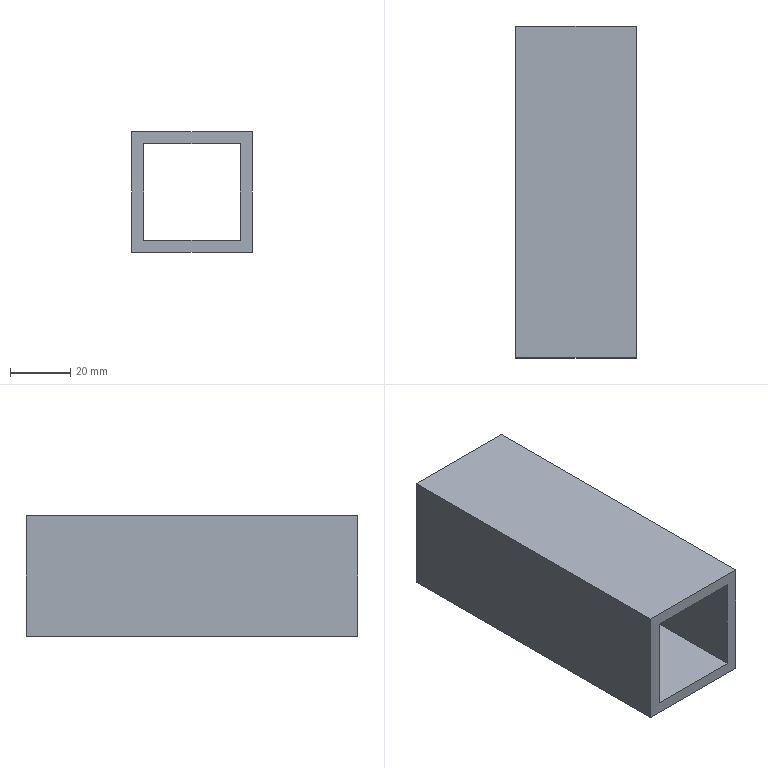Part | NX | features solid 2 | 1 solid | 10 faces | box 40 x 110 x 40 mm | volume 63360 mm3 | plane 10
STEP:
#1=CARTESIAN_POINT('',(1100.,-330.,-85.));
#2=VERTEX_POINT('',#1);
#3=CARTESIAN_POINT('',(1100.,-220.,-85.));
#4=VERTEX_POINT('',#3);
#5=CARTESIAN_POINT('',(1100.,1629.393,-85.));
#6=DIRECTION('',(0.,1.,0.));
#7=VECTOR('',#6,1000.);
#8=LINE('',#5,#7);
#9=EDGE_CURVE('',#2,#4,#8,.T.);
#10=ORIENTED_EDGE('',*,*,#9,.F.);
#11=CARTESIAN_POINT('',(1100.,-330.,-45.));
#12=VERTEX_POINT('',#11);
#13=CARTESIAN_POINT('',(1100.,-330.,-70.));
#14=DIRECTION('',(0.,0.,1.));
#15=VECTOR('',#14,1000.);
#16=LINE('',#13,#15);
#17=EDGE_CURVE('',#2,#12,#16,.T.);
#18=ORIENTED_EDGE('',*,*,#17,.T.);
#19=CARTESIAN_POINT('',(1100.,-220.,-45.));
#20=VERTEX_POINT('',#19);
#21=CARTESIAN_POINT('',(1100.,1714.393,-45.));
#22=DIRECTION('',(0.,1.,0.));
#23=VECTOR('',#22,1000.);
#24=LINE('',#21,#23);
#25=EDGE_CURVE('',#12,#20,#24,.T.);
#26=ORIENTED_EDGE('',*,*,#25,.T.);
#27=CARTESIAN_POINT('',(1100.,-220.,-70.));
#28=DIRECTION('',(0.,0.,1.));
#29=VECTOR('',#28,1000.);
#30=LINE('',#27,#29);
#31=EDGE_CURVE('',#4,#20,#30,.T.);
#32=ORIENTED_EDGE('',*,*,#31,.F.);
#33=EDGE_LOOP('',(#10,#18,#26,#32));
#34=FACE_BOUND('',#33,.T.);
#35=CARTESIAN_POINT('',(1100.,1629.393,-70.));
#36=DIRECTION('',(1.,0.,0.));
#37=DIRECTION('',(0.,0.,1.));
#38=AXIS2_PLACEMENT_3D('',#35,#36,#37);
#39=PLANE('',#38);
#40=ADVANCED_FACE('',(#34),#39,.F.);
#41=CARTESIAN_POINT('',(1140.,-330.,-85.));
#42=VERTEX_POINT('',#41);
#43=CARTESIAN_POINT('',(1140.,-220.,-85.));
#44=VERTEX_POINT('',#43);
#45=CARTESIAN_POINT('',(1140.,1714.393,-85.));
#46=DIRECTION('',(0.,1.,0.));
#47=VECTOR('',#46,1000.);
#48=LINE('',#45,#47);
#49=EDGE_CURVE('',#42,#44,#48,.T.);
#50=ORIENTED_EDGE('',*,*,#49,.F.);
#51=CARTESIAN_POINT('',(520.,-330.,-85.));
#52=DIRECTION('',(-1.,0.,0.));
#53=VECTOR('',#52,1000.);
#54=LINE('',#51,#53);
#55=EDGE_CURVE('',#42,#2,#54,.T.);
#56=ORIENTED_EDGE('',*,*,#55,.T.);
#57=ORIENTED_EDGE('',*,*,#9,.T.);
#58=CARTESIAN_POINT('',(520.,-220.,-85.));
#59=DIRECTION('',(-1.,0.,0.));
#60=VECTOR('',#59,1000.);
#61=LINE('',#58,#60);
#62=EDGE_CURVE('',#44,#4,#61,.T.);
#63=ORIENTED_EDGE('',*,*,#62,.F.);
#64=EDGE_LOOP('',(#50,#56,#57,#63));
#65=FACE_BOUND('',#64,.T.);
#66=CARTESIAN_POINT('',(520.,1714.393,-85.));
#67=DIRECTION('',(0.,0.,1.));
#68=DIRECTION('',(-1.,0.,0.));
#69=AXIS2_PLACEMENT_3D('',#66,#67,#68);
#70=PLANE('',#69);
#71=ADVANCED_FACE('',(#65),#70,.F.);
#72=ORIENTED_EDGE('',*,*,#25,.F.);
#73=CARTESIAN_POINT('',(1140.,-330.,-45.));
#74=VERTEX_POINT('',#73);
#75=CARTESIAN_POINT('',(480.,-330.,-45.));
#76=DIRECTION('',(1.,0.,0.));
#77=VECTOR('',#76,1000.);
#78=LINE('',#75,#77);
#79=EDGE_CURVE('',#12,#74,#78,.T.);
#80=ORIENTED_EDGE('',*,*,#79,.T.);
#81=CARTESIAN_POINT('',(1140.,-220.,-45.));
#82=VERTEX_POINT('',#81);
#83=CARTESIAN_POINT('',(1140.,1714.393,-45.));
#84=DIRECTION('',(0.,-1.,0.));
#85=VECTOR('',#84,1000.);
#86=LINE('',#83,#85);
#87=EDGE_CURVE('',#82,#74,#86,.T.);
#88=ORIENTED_EDGE('',*,*,#87,.F.);
#89=CARTESIAN_POINT('',(480.,-220.,-45.));
#90=DIRECTION('',(1.,0.,0.));
#91=VECTOR('',#90,1000.);
#92=LINE('',#89,#91);
#93=EDGE_CURVE('',#20,#82,#92,.T.);
#94=ORIENTED_EDGE('',*,*,#93,.F.);
#95=EDGE_LOOP('',(#72,#80,#88,#94));
#96=FACE_BOUND('',#95,.T.);
#97=CARTESIAN_POINT('',(480.,1714.393,-45.));
#98=DIRECTION('',(0.,0.,-1.));
#99=DIRECTION('',(1.,0.,0.));
#100=AXIS2_PLACEMENT_3D('',#97,#98,#99);
#101=PLANE('',#100);
#102=ADVANCED_FACE('',(#96),#101,.F.);
#103=ORIENTED_EDGE('',*,*,#87,.T.);
#104=CARTESIAN_POINT('',(1140.,-330.,-40.));
#105=DIRECTION('',(0.,0.,-1.));
#106=VECTOR('',#105,1000.);
#107=LINE('',#104,#106);
#108=EDGE_CURVE('',#74,#42,#107,.T.);
#109=ORIENTED_EDGE('',*,*,#108,.T.);
#110=ORIENTED_EDGE('',*,*,#49,.T.);
#111=CARTESIAN_POINT('',(1140.,-220.,-40.));
#112=DIRECTION('',(0.,0.,-1.));
#113=VECTOR('',#112,1000.);
#114=LINE('',#111,#113);
#115=EDGE_CURVE('',#82,#44,#114,.T.);
#116=ORIENTED_EDGE('',*,*,#115,.F.);
#117=EDGE_LOOP('',(#103,#109,#110,#116));
#118=FACE_BOUND('',#117,.T.);
#119=CARTESIAN_POINT('',(1140.,1629.393,-40.));
#120=DIRECTION('',(-1.,0.,0.));
#121=DIRECTION('',(0.,0.,-1.));
#122=AXIS2_PLACEMENT_3D('',#119,#120,#121);
#123=PLANE('',#122);
#124=ADVANCED_FACE('',(#118),#123,.F.);
#125=CARTESIAN_POINT('',(1104.,-330.,-81.));
#126=VERTEX_POINT('',#125);
#127=CARTESIAN_POINT('',(1104.,-330.,-49.));
#128=VERTEX_POINT('',#127);
#129=CARTESIAN_POINT('',(1104.,-330.,-70.));
#130=DIRECTION('',(0.,0.,1.));
#131=VECTOR('',#130,1000.);
#132=LINE('',#129,#131);
#133=EDGE_CURVE('',#126,#128,#132,.T.);
#134=ORIENTED_EDGE('',*,*,#133,.T.);
#135=CARTESIAN_POINT('',(1136.,-330.,-49.));
#136=VERTEX_POINT('',#135);
#137=CARTESIAN_POINT('',(480.,-330.,-49.));
#138=DIRECTION('',(1.,0.,0.));
#139=VECTOR('',#138,1000.);
#140=LINE('',#137,#139);
#141=EDGE_CURVE('',#128,#136,#140,.T.);
#142=ORIENTED_EDGE('',*,*,#141,.T.);
#143=CARTESIAN_POINT('',(1136.,-330.,-81.));
#144=VERTEX_POINT('',#143);
#145=CARTESIAN_POINT('',(1136.,-330.,-40.));
#146=DIRECTION('',(0.,0.,-1.));
#147=VECTOR('',#146,1000.);
#148=LINE('',#145,#147);
#149=EDGE_CURVE('',#136,#144,#148,.T.);
#150=ORIENTED_EDGE('',*,*,#149,.T.);
#151=CARTESIAN_POINT('',(520.,-330.,-81.));
#152=DIRECTION('',(-1.,0.,0.));
#153=VECTOR('',#152,1000.);
#154=LINE('',#151,#153);
#155=EDGE_CURVE('',#144,#126,#154,.T.);
#156=ORIENTED_EDGE('',*,*,#155,.T.);
#157=EDGE_LOOP('',(#134,#142,#150,#156));
#158=FACE_BOUND('',#157,.T.);
#159=ORIENTED_EDGE('',*,*,#55,.F.);
#160=ORIENTED_EDGE('',*,*,#108,.F.);
#161=ORIENTED_EDGE('',*,*,#79,.F.);
#162=ORIENTED_EDGE('',*,*,#17,.F.);
#163=EDGE_LOOP('',(#159,#160,#161,#162));
#164=FACE_BOUND('',#163,.T.);
#165=CARTESIAN_POINT('',(1250.,-330.,-45.));
#166=DIRECTION('',(0.,-1.,0.));
#167=DIRECTION('',(0.,0.,-1.));
#168=AXIS2_PLACEMENT_3D('',#165,#166,#167);
#169=PLANE('',#168);
#170=ADVANCED_FACE('',(#158,#164),#169,.T.);
#171=CARTESIAN_POINT('',(1104.,-220.,-81.));
#172=VERTEX_POINT('',#171);
#173=CARTESIAN_POINT('',(1104.,-220.,-49.));
#174=VERTEX_POINT('',#173);
#175=CARTESIAN_POINT('',(1104.,-220.,-70.));
#176=DIRECTION('',(0.,0.,1.));
#177=VECTOR('',#176,1000.);
#178=LINE('',#175,#177);
#179=EDGE_CURVE('',#172,#174,#178,.T.);
#180=ORIENTED_EDGE('',*,*,#179,.T.);
#181=CARTESIAN_POINT('',(1104.,1714.393,-49.));
#182=DIRECTION('',(0.,1.,0.));
#183=VECTOR('',#182,1000.);
#184=LINE('',#181,#183);
#185=EDGE_CURVE('',#128,#174,#184,.T.);
#186=ORIENTED_EDGE('',*,*,#185,.F.);
#187=ORIENTED_EDGE('',*,*,#133,.F.);
#188=CARTESIAN_POINT('',(1104.,1629.393,-81.));
#189=DIRECTION('',(0.,1.,0.));
#190=VECTOR('',#189,1000.);
#191=LINE('',#188,#190);
#192=EDGE_CURVE('',#126,#172,#191,.T.);
#193=ORIENTED_EDGE('',*,*,#192,.T.);
#194=EDGE_LOOP('',(#180,#186,#187,#193));
#195=FACE_BOUND('',#194,.T.);
#196=CARTESIAN_POINT('',(1104.,1629.393,-70.));
#197=DIRECTION('',(1.,0.,0.));
#198=DIRECTION('',(0.,0.,1.));
#199=AXIS2_PLACEMENT_3D('',#196,#197,#198);
#200=PLANE('',#199);
#201=ADVANCED_FACE('',(#195),#200,.T.);
#202=CARTESIAN_POINT('',(1136.,-220.,-81.));
#203=VERTEX_POINT('',#202);
#204=CARTESIAN_POINT('',(520.,-220.,-81.));
#205=DIRECTION('',(-1.,0.,0.));
#206=VECTOR('',#205,1000.);
#207=LINE('',#204,#206);
#208=EDGE_CURVE('',#203,#172,#207,.T.);
#209=ORIENTED_EDGE('',*,*,#208,.T.);
#210=ORIENTED_EDGE('',*,*,#192,.F.);
#211=ORIENTED_EDGE('',*,*,#155,.F.);
#212=CARTESIAN_POINT('',(1136.,1714.393,-81.));
#213=DIRECTION('',(0.,1.,0.));
#214=VECTOR('',#213,1000.);
#215=LINE('',#212,#214);
#216=EDGE_CURVE('',#144,#203,#215,.T.);
#217=ORIENTED_EDGE('',*,*,#216,.T.);
#218=EDGE_LOOP('',(#209,#210,#211,#217));
#219=FACE_BOUND('',#218,.T.);
#220=CARTESIAN_POINT('',(520.,1714.393,-81.));
#221=DIRECTION('',(0.,0.,1.));
#222=DIRECTION('',(-1.,0.,0.));
#223=AXIS2_PLACEMENT_3D('',#220,#221,#222);
#224=PLANE('',#223);
#225=ADVANCED_FACE('',(#219),#224,.T.);
#226=CARTESIAN_POINT('',(1136.,-220.,-49.));
#227=VERTEX_POINT('',#226);
#228=CARTESIAN_POINT('',(480.,-220.,-49.));
#229=DIRECTION('',(1.,0.,0.));
#230=VECTOR('',#229,1000.);
#231=LINE('',#228,#230);
#232=EDGE_CURVE('',#174,#227,#231,.T.);
#233=ORIENTED_EDGE('',*,*,#232,.T.);
#234=CARTESIAN_POINT('',(1136.,1714.393,-49.));
#235=DIRECTION('',(0.,-1.,0.));
#236=VECTOR('',#235,1000.);
#237=LINE('',#234,#236);
#238=EDGE_CURVE('',#227,#136,#237,.T.);
#239=ORIENTED_EDGE('',*,*,#238,.T.);
#240=ORIENTED_EDGE('',*,*,#141,.F.);
#241=ORIENTED_EDGE('',*,*,#185,.T.);
#242=EDGE_LOOP('',(#233,#239,#240,#241));
#243=FACE_BOUND('',#242,.T.);
#244=CARTESIAN_POINT('',(480.,1714.393,-49.));
#245=DIRECTION('',(0.,0.,-1.));
#246=DIRECTION('',(1.,0.,0.));
#247=AXIS2_PLACEMENT_3D('',#244,#245,#246);
#248=PLANE('',#247);
#249=ADVANCED_FACE('',(#243),#248,.T.);
#250=CARTESIAN_POINT('',(1136.,-220.,-40.));
#251=DIRECTION('',(0.,0.,-1.));
#252=VECTOR('',#251,1000.);
#253=LINE('',#250,#252);
#254=EDGE_CURVE('',#227,#203,#253,.T.);
#255=ORIENTED_EDGE('',*,*,#254,.T.);
#256=ORIENTED_EDGE('',*,*,#216,.F.);
#257=ORIENTED_EDGE('',*,*,#149,.F.);
#258=ORIENTED_EDGE('',*,*,#238,.F.);
#259=EDGE_LOOP('',(#255,#256,#257,#258));
#260=FACE_BOUND('',#259,.T.);
#261=CARTESIAN_POINT('',(1136.,1629.393,-40.));
#262=DIRECTION('',(-1.,0.,0.));
#263=DIRECTION('',(0.,0.,-1.));
#264=AXIS2_PLACEMENT_3D('',#261,#262,#263);
#265=PLANE('',#264);
#266=ADVANCED_FACE('',(#260),#265,.T.);
#267=ORIENTED_EDGE('',*,*,#179,.F.);
#268=ORIENTED_EDGE('',*,*,#208,.F.);
#269=ORIENTED_EDGE('',*,*,#254,.F.);
#270=ORIENTED_EDGE('',*,*,#232,.F.);
#271=EDGE_LOOP('',(#267,#268,#269,#270));
#272=FACE_BOUND('',#271,.T.);
#273=ORIENTED_EDGE('',*,*,#62,.T.);
#274=ORIENTED_EDGE('',*,*,#31,.T.);
#275=ORIENTED_EDGE('',*,*,#93,.T.);
#276=ORIENTED_EDGE('',*,*,#115,.T.);
#277=EDGE_LOOP('',(#273,#274,#275,#276));
#278=FACE_BOUND('',#277,.T.);
#279=CARTESIAN_POINT('',(1100.,-220.,-45.));
#280=DIRECTION('',(0.,-1.,0.));
#281=DIRECTION('',(0.,0.,-1.));
#282=AXIS2_PLACEMENT_3D('',#279,#280,#281);
#283=PLANE('',#282);
#284=ADVANCED_FACE('',(#272,#278),#283,.F.);
#285=CLOSED_SHELL('',(#40,#71,#102,#124,#170,#201,#225,#249,#266,#284));
#286=MANIFOLD_SOLID_BREP('',#285);
#287=(LENGTH_UNIT()NAMED_UNIT(*)SI_UNIT(.MILLI.,.METRE.));
#288=UNCERTAINTY_MEASURE_WITH_UNIT(LENGTH_MEASURE(0.00001),#287,'','');
#289=(NAMED_UNIT(*)PLANE_ANGLE_UNIT()SI_UNIT($,.RADIAN.));
#290=(NAMED_UNIT(*)SI_UNIT($,.STERADIAN.)SOLID_ANGLE_UNIT());
#291=(GEOMETRIC_REPRESENTATION_CONTEXT(3)GLOBAL_UNCERTAINTY_ASSIGNED_CONTEXT((#288))GLOBAL_UNIT_ASSIGNED_CONTEXT((#287,#289,#290))REPRESENTATION_CONTEXT('',''));
#292=ADVANCED_BREP_SHAPE_REPRESENTATION('',(#286),#291);